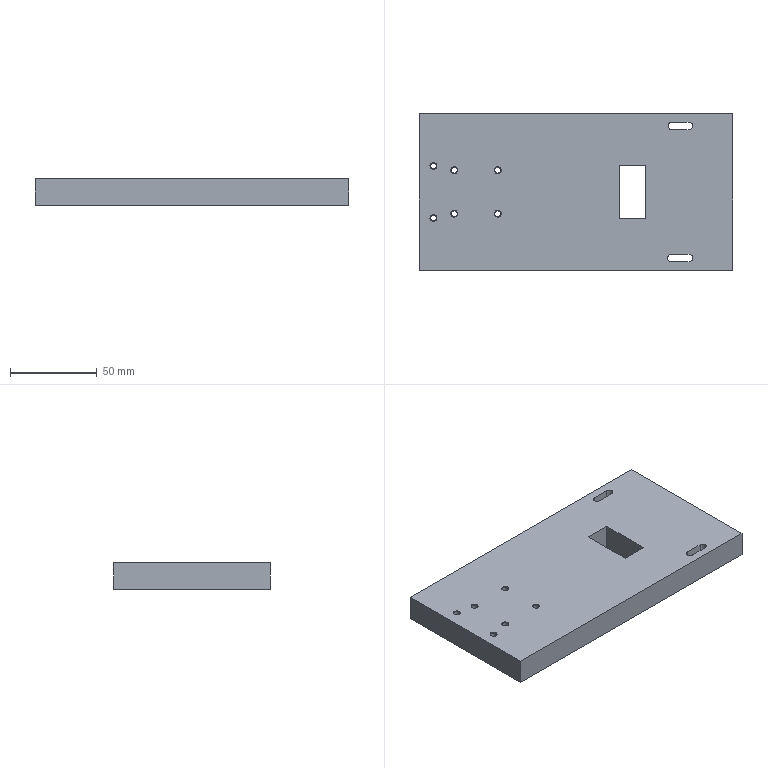Part | NX | features SIMPLE HOLE 6, SYMBOLIC_THREAD 6, DATUM_CSYS 5, SKETCH 4, EXTRUDE 3, HOLE PACKAGE 1 | 1 solid | 36 faces | box 180 x 90 x 15 mm | volume 233788 mm3 | plane 14 | cone 12 | cylinder 10 | commonest cylinder face diameters 3.3 x6 4.2 x4
STEP:
#1=CARTESIAN_POINT('',(-90.,45.,0.));
#2=VERTEX_POINT('',#1);
#3=CARTESIAN_POINT('',(-90.,-45.,0.));
#4=VERTEX_POINT('',#3);
#5=CARTESIAN_POINT('',(-90.,45.,0.));
#6=DIRECTION('',(0.,-1.,0.));
#7=VECTOR('',#6,1000.);
#8=LINE('',#5,#7);
#9=EDGE_CURVE('',#2,#4,#8,.T.);
#10=ORIENTED_EDGE('',*,*,#9,.T.);
#11=CARTESIAN_POINT('',(-90.,-45.,15.));
#12=VERTEX_POINT('',#11);
#13=CARTESIAN_POINT('',(-90.,-45.,15.));
#14=DIRECTION('',(0.,0.,-1.));
#15=VECTOR('',#14,1000.);
#16=LINE('',#13,#15);
#17=EDGE_CURVE('',#12,#4,#16,.T.);
#18=ORIENTED_EDGE('',*,*,#17,.F.);
#19=CARTESIAN_POINT('',(-90.,45.,15.));
#20=VERTEX_POINT('',#19);
#21=CARTESIAN_POINT('',(-90.,45.,15.));
#22=DIRECTION('',(0.,-1.,0.));
#23=VECTOR('',#22,1000.);
#24=LINE('',#21,#23);
#25=EDGE_CURVE('',#20,#12,#24,.T.);
#26=ORIENTED_EDGE('',*,*,#25,.F.);
#27=CARTESIAN_POINT('',(-90.,45.,15.));
#28=DIRECTION('',(0.,0.,-1.));
#29=VECTOR('',#28,1000.);
#30=LINE('',#27,#29);
#31=EDGE_CURVE('',#20,#2,#30,.T.);
#32=ORIENTED_EDGE('',*,*,#31,.T.);
#33=EDGE_LOOP('',(#10,#18,#26,#32));
#34=FACE_BOUND('',#33,.T.);
#35=CARTESIAN_POINT('',(-90.,45.,15.));
#36=DIRECTION('',(1.,0.,0.));
#37=DIRECTION('',(0.,0.,-1.));
#38=AXIS2_PLACEMENT_3D('',#35,#36,#37);
#39=PLANE('',#38);
#40=ADVANCED_FACE('',(#34),#39,.F.);
#41=CARTESIAN_POINT('',(90.,-45.,0.));
#42=VERTEX_POINT('',#41);
#43=CARTESIAN_POINT('',(-90.,-45.,0.));
#44=DIRECTION('',(1.,0.,0.));
#45=VECTOR('',#44,1000.);
#46=LINE('',#43,#45);
#47=EDGE_CURVE('',#4,#42,#46,.T.);
#48=ORIENTED_EDGE('',*,*,#47,.T.);
#49=CARTESIAN_POINT('',(90.,-45.,15.));
#50=VERTEX_POINT('',#49);
#51=CARTESIAN_POINT('',(90.,-45.,15.));
#52=DIRECTION('',(0.,0.,-1.));
#53=VECTOR('',#52,1000.);
#54=LINE('',#51,#53);
#55=EDGE_CURVE('',#50,#42,#54,.T.);
#56=ORIENTED_EDGE('',*,*,#55,.F.);
#57=CARTESIAN_POINT('',(-90.,-45.,15.));
#58=DIRECTION('',(1.,0.,0.));
#59=VECTOR('',#58,1000.);
#60=LINE('',#57,#59);
#61=EDGE_CURVE('',#12,#50,#60,.T.);
#62=ORIENTED_EDGE('',*,*,#61,.F.);
#63=ORIENTED_EDGE('',*,*,#17,.T.);
#64=EDGE_LOOP('',(#48,#56,#62,#63));
#65=FACE_BOUND('',#64,.T.);
#66=CARTESIAN_POINT('',(-90.,-45.,15.));
#67=DIRECTION('',(0.,1.,0.));
#68=DIRECTION('',(0.,0.,1.));
#69=AXIS2_PLACEMENT_3D('',#66,#67,#68);
#70=PLANE('',#69);
#71=ADVANCED_FACE('',(#65),#70,.F.);
#72=CARTESIAN_POINT('',(90.,45.,0.));
#73=VERTEX_POINT('',#72);
#74=CARTESIAN_POINT('',(90.,-45.,0.));
#75=DIRECTION('',(0.,1.,0.));
#76=VECTOR('',#75,1000.);
#77=LINE('',#74,#76);
#78=EDGE_CURVE('',#42,#73,#77,.T.);
#79=ORIENTED_EDGE('',*,*,#78,.T.);
#80=CARTESIAN_POINT('',(90.,45.,15.));
#81=VERTEX_POINT('',#80);
#82=CARTESIAN_POINT('',(90.,45.,15.));
#83=DIRECTION('',(0.,0.,-1.));
#84=VECTOR('',#83,1000.);
#85=LINE('',#82,#84);
#86=EDGE_CURVE('',#81,#73,#85,.T.);
#87=ORIENTED_EDGE('',*,*,#86,.F.);
#88=CARTESIAN_POINT('',(90.,-45.,15.));
#89=DIRECTION('',(0.,1.,0.));
#90=VECTOR('',#89,1000.);
#91=LINE('',#88,#90);
#92=EDGE_CURVE('',#50,#81,#91,.T.);
#93=ORIENTED_EDGE('',*,*,#92,.F.);
#94=ORIENTED_EDGE('',*,*,#55,.T.);
#95=EDGE_LOOP('',(#79,#87,#93,#94));
#96=FACE_BOUND('',#95,.T.);
#97=CARTESIAN_POINT('',(90.,-45.,15.));
#98=DIRECTION('',(-1.,0.,0.));
#99=DIRECTION('',(0.,0.,1.));
#100=AXIS2_PLACEMENT_3D('',#97,#98,#99);
#101=PLANE('',#100);
#102=ADVANCED_FACE('',(#96),#101,.F.);
#103=CARTESIAN_POINT('',(90.,45.,0.));
#104=DIRECTION('',(-1.,0.,0.));
#105=VECTOR('',#104,1000.);
#106=LINE('',#103,#105);
#107=EDGE_CURVE('',#73,#2,#106,.T.);
#108=ORIENTED_EDGE('',*,*,#107,.T.);
#109=ORIENTED_EDGE('',*,*,#31,.F.);
#110=CARTESIAN_POINT('',(90.,45.,15.));
#111=DIRECTION('',(-1.,0.,0.));
#112=VECTOR('',#111,1000.);
#113=LINE('',#110,#112);
#114=EDGE_CURVE('',#81,#20,#113,.T.);
#115=ORIENTED_EDGE('',*,*,#114,.F.);
#116=ORIENTED_EDGE('',*,*,#86,.T.);
#117=EDGE_LOOP('',(#108,#109,#115,#116));
#118=FACE_BOUND('',#117,.T.);
#119=CARTESIAN_POINT('',(90.,45.,15.));
#120=DIRECTION('',(0.,-1.,0.));
#121=DIRECTION('',(0.,0.,-1.));
#122=AXIS2_PLACEMENT_3D('',#119,#120,#121);
#123=PLANE('',#122);
#124=ADVANCED_FACE('',(#118),#123,.F.);
#125=CARTESIAN_POINT('',(25.,15.,15.));
#126=VERTEX_POINT('',#125);
#127=CARTESIAN_POINT('',(25.,-15.,15.));
#128=VERTEX_POINT('',#127);
#129=CARTESIAN_POINT('',(25.,15.,15.));
#130=DIRECTION('',(0.,-1.,0.));
#131=VECTOR('',#130,1000.);
#132=LINE('',#129,#131);
#133=EDGE_CURVE('',#126,#128,#132,.T.);
#134=ORIENTED_EDGE('',*,*,#133,.F.);
#135=CARTESIAN_POINT('',(40.,15.,15.));
#136=VERTEX_POINT('',#135);
#137=CARTESIAN_POINT('',(40.,15.,15.));
#138=DIRECTION('',(-1.,0.,0.));
#139=VECTOR('',#138,1000.);
#140=LINE('',#137,#139);
#141=EDGE_CURVE('',#136,#126,#140,.T.);
#142=ORIENTED_EDGE('',*,*,#141,.F.);
#143=CARTESIAN_POINT('',(40.,-15.,15.));
#144=VERTEX_POINT('',#143);
#145=CARTESIAN_POINT('',(40.,-15.,15.));
#146=DIRECTION('',(0.,1.,0.));
#147=VECTOR('',#146,1000.);
#148=LINE('',#145,#147);
#149=EDGE_CURVE('',#144,#136,#148,.T.);
#150=ORIENTED_EDGE('',*,*,#149,.F.);
#151=CARTESIAN_POINT('',(25.,-15.,15.));
#152=DIRECTION('',(1.,0.,0.));
#153=VECTOR('',#152,1000.);
#154=LINE('',#151,#153);
#155=EDGE_CURVE('',#128,#144,#154,.T.);
#156=ORIENTED_EDGE('',*,*,#155,.F.);
#157=EDGE_LOOP('',(#134,#142,#150,#156));
#158=FACE_BOUND('',#157,.T.);
#159=CARTESIAN_POINT('',(-80.,15.,15.));
#160=VERTEX_POINT('',#159);
#161=CARTESIAN_POINT('',(-82.,15.,15.));
#162=DIRECTION('',(0.,0.,1.));
#163=DIRECTION('',(1.,0.,0.));
#164=AXIS2_PLACEMENT_3D('',#161,#162,#163);
#165=CIRCLE('',#164,2.);
#166=EDGE_CURVE('',#160,#160,#165,.F.);
#167=ORIENTED_EDGE('',*,*,#166,.T.);
#168=EDGE_LOOP('',(#167));
#169=FACE_BOUND('',#168,.T.);
#170=CARTESIAN_POINT('',(-80.,-15.,15.));
#171=VERTEX_POINT('',#170);
#172=CARTESIAN_POINT('',(-82.,-15.,15.));
#173=DIRECTION('',(0.,0.,1.));
#174=DIRECTION('',(1.,0.,0.));
#175=AXIS2_PLACEMENT_3D('',#172,#173,#174);
#176=CIRCLE('',#175,2.);
#177=EDGE_CURVE('',#171,#171,#176,.F.);
#178=ORIENTED_EDGE('',*,*,#177,.T.);
#179=EDGE_LOOP('',(#178));
#180=FACE_BOUND('',#179,.T.);
#181=CARTESIAN_POINT('',(-43.,12.5,15.));
#182=VERTEX_POINT('',#181);
#183=CARTESIAN_POINT('',(-45.,12.5,15.));
#184=DIRECTION('',(0.,0.,1.));
#185=DIRECTION('',(1.,0.,0.));
#186=AXIS2_PLACEMENT_3D('',#183,#184,#185);
#187=CIRCLE('',#186,2.);
#188=EDGE_CURVE('',#182,#182,#187,.F.);
#189=ORIENTED_EDGE('',*,*,#188,.T.);
#190=EDGE_LOOP('',(#189));
#191=FACE_BOUND('',#190,.T.);
#192=CARTESIAN_POINT('',(-43.,-12.5,15.));
#193=VERTEX_POINT('',#192);
#194=CARTESIAN_POINT('',(-45.,-12.5,15.));
#195=DIRECTION('',(0.,0.,1.));
#196=DIRECTION('',(1.,0.,0.));
#197=AXIS2_PLACEMENT_3D('',#194,#195,#196);
#198=CIRCLE('',#197,2.);
#199=EDGE_CURVE('',#193,#193,#198,.F.);
#200=ORIENTED_EDGE('',*,*,#199,.T.);
#201=EDGE_LOOP('',(#200));
#202=FACE_BOUND('',#201,.T.);
#203=CARTESIAN_POINT('',(-68.,12.5,15.));
#204=VERTEX_POINT('',#203);
#205=CARTESIAN_POINT('',(-70.,12.5,15.));
#206=DIRECTION('',(0.,0.,1.));
#207=DIRECTION('',(1.,0.,0.));
#208=AXIS2_PLACEMENT_3D('',#205,#206,#207);
#209=CIRCLE('',#208,2.);
#210=EDGE_CURVE('',#204,#204,#209,.F.);
#211=ORIENTED_EDGE('',*,*,#210,.T.);
#212=EDGE_LOOP('',(#211));
#213=FACE_BOUND('',#212,.T.);
#214=CARTESIAN_POINT('',(-68.,-12.5,15.));
#215=VERTEX_POINT('',#214);
#216=CARTESIAN_POINT('',(-70.,-12.5,15.));
#217=DIRECTION('',(0.,0.,1.));
#218=DIRECTION('',(1.,0.,0.));
#219=AXIS2_PLACEMENT_3D('',#216,#217,#218);
#220=CIRCLE('',#219,2.);
#221=EDGE_CURVE('',#215,#215,#220,.F.);
#222=ORIENTED_EDGE('',*,*,#221,.T.);
#223=EDGE_LOOP('',(#222));
#224=FACE_BOUND('',#223,.T.);
#225=CARTESIAN_POINT('',(55.,40.1,15.));
#226=VERTEX_POINT('',#225);
#227=CARTESIAN_POINT('',(55.,35.9,15.));
#228=VERTEX_POINT('',#227);
#229=CARTESIAN_POINT('',(55.,38.,15.));
#230=DIRECTION('',(0.,0.,1.));
#231=DIRECTION('',(0.,1.,0.));
#232=AXIS2_PLACEMENT_3D('',#229,#230,#231);
#233=CIRCLE('',#232,2.1);
#234=EDGE_CURVE('',#226,#228,#233,.T.);
#235=ORIENTED_EDGE('',*,*,#234,.F.);
#236=CARTESIAN_POINT('',(65.,40.1,15.));
#237=VERTEX_POINT('',#236);
#238=CARTESIAN_POINT('',(65.,40.1,15.));
#239=DIRECTION('',(-1.,0.,0.));
#240=VECTOR('',#239,1000.);
#241=LINE('',#238,#240);
#242=EDGE_CURVE('',#237,#226,#241,.T.);
#243=ORIENTED_EDGE('',*,*,#242,.F.);
#244=CARTESIAN_POINT('',(65.,35.9,15.));
#245=VERTEX_POINT('',#244);
#246=CARTESIAN_POINT('',(65.,38.,15.));
#247=DIRECTION('',(0.,0.,1.));
#248=DIRECTION('',(0.,1.,0.));
#249=AXIS2_PLACEMENT_3D('',#246,#247,#248);
#250=CIRCLE('',#249,2.1);
#251=EDGE_CURVE('',#245,#237,#250,.T.);
#252=ORIENTED_EDGE('',*,*,#251,.F.);
#253=CARTESIAN_POINT('',(55.,35.9,15.));
#254=DIRECTION('',(1.,0.,0.));
#255=VECTOR('',#254,1000.);
#256=LINE('',#253,#255);
#257=EDGE_CURVE('',#228,#245,#256,.T.);
#258=ORIENTED_EDGE('',*,*,#257,.F.);
#259=EDGE_LOOP('',(#235,#243,#252,#258));
#260=FACE_BOUND('',#259,.T.);
#261=CARTESIAN_POINT('',(54.858,-35.9,15.));
#262=VERTEX_POINT('',#261);
#263=CARTESIAN_POINT('',(54.858,-40.1,15.));
#264=VERTEX_POINT('',#263);
#265=CARTESIAN_POINT('',(54.858,-38.,15.));
#266=DIRECTION('',(0.,0.,1.));
#267=DIRECTION('',(0.,1.,0.));
#268=AXIS2_PLACEMENT_3D('',#265,#266,#267);
#269=CIRCLE('',#268,2.1);
#270=EDGE_CURVE('',#262,#264,#269,.T.);
#271=ORIENTED_EDGE('',*,*,#270,.F.);
#272=CARTESIAN_POINT('',(65.,-35.9,15.));
#273=VERTEX_POINT('',#272);
#274=CARTESIAN_POINT('',(65.,-35.9,15.));
#275=DIRECTION('',(-1.,0.,0.));
#276=VECTOR('',#275,1000.);
#277=LINE('',#274,#276);
#278=EDGE_CURVE('',#273,#262,#277,.T.);
#279=ORIENTED_EDGE('',*,*,#278,.F.);
#280=CARTESIAN_POINT('',(65.,-40.1,15.));
#281=VERTEX_POINT('',#280);
#282=CARTESIAN_POINT('',(65.,-38.,15.));
#283=DIRECTION('',(0.,0.,1.));
#284=DIRECTION('',(0.,1.,0.));
#285=AXIS2_PLACEMENT_3D('',#282,#283,#284);
#286=CIRCLE('',#285,2.1);
#287=EDGE_CURVE('',#281,#273,#286,.T.);
#288=ORIENTED_EDGE('',*,*,#287,.F.);
#289=CARTESIAN_POINT('',(54.858,-40.1,15.));
#290=DIRECTION('',(1.,0.,0.));
#291=VECTOR('',#290,1000.);
#292=LINE('',#289,#291);
#293=EDGE_CURVE('',#264,#281,#292,.T.);
#294=ORIENTED_EDGE('',*,*,#293,.F.);
#295=EDGE_LOOP('',(#271,#279,#288,#294));
#296=FACE_BOUND('',#295,.T.);
#297=ORIENTED_EDGE('',*,*,#25,.T.);
#298=ORIENTED_EDGE('',*,*,#61,.T.);
#299=ORIENTED_EDGE('',*,*,#92,.T.);
#300=ORIENTED_EDGE('',*,*,#114,.T.);
#301=EDGE_LOOP('',(#297,#298,#299,#300));
#302=FACE_BOUND('',#301,.T.);
#303=CARTESIAN_POINT('',(0.,0.,15.));
#304=DIRECTION('',(0.,0.,1.));
#305=DIRECTION('',(1.,0.,0.));
#306=AXIS2_PLACEMENT_3D('',#303,#304,#305);
#307=PLANE('',#306);
#308=ADVANCED_FACE('',(#158,#169,#180,#191,#202,#213,#224,#260,#296,#302),#307,.T.);
#309=CARTESIAN_POINT('',(40.,15.,0.));
#310=VERTEX_POINT('',#309);
#311=CARTESIAN_POINT('',(25.,15.,0.));
#312=VERTEX_POINT('',#311);
#313=CARTESIAN_POINT('',(40.,15.,0.));
#314=DIRECTION('',(-1.,0.,0.));
#315=VECTOR('',#314,1000.);
#316=LINE('',#313,#315);
#317=EDGE_CURVE('',#310,#312,#316,.T.);
#318=ORIENTED_EDGE('',*,*,#317,.T.);
#319=CARTESIAN_POINT('',(25.,-15.,0.));
#320=VERTEX_POINT('',#319);
#321=CARTESIAN_POINT('',(25.,15.,0.));
#322=DIRECTION('',(0.,-1.,0.));
#323=VECTOR('',#322,1000.);
#324=LINE('',#321,#323);
#325=EDGE_CURVE('',#312,#320,#324,.T.);
#326=ORIENTED_EDGE('',*,*,#325,.T.);
#327=CARTESIAN_POINT('',(40.,-15.,0.));
#328=VERTEX_POINT('',#327);
#329=CARTESIAN_POINT('',(25.,-15.,0.));
#330=DIRECTION('',(1.,0.,0.));
#331=VECTOR('',#330,1000.);
#332=LINE('',#329,#331);
#333=EDGE_CURVE('',#320,#328,#332,.T.);
#334=ORIENTED_EDGE('',*,*,#333,.T.);
#335=CARTESIAN_POINT('',(40.,-15.,0.));
#336=DIRECTION('',(0.,1.,0.));
#337=VECTOR('',#336,1000.);
#338=LINE('',#335,#337);
#339=EDGE_CURVE('',#328,#310,#338,.T.);
#340=ORIENTED_EDGE('',*,*,#339,.T.);
#341=EDGE_LOOP('',(#318,#326,#334,#340));
#342=FACE_BOUND('',#341,.T.);
#343=CARTESIAN_POINT('',(-80.,15.,0.));
#344=VERTEX_POINT('',#343);
#345=CARTESIAN_POINT('',(-82.,15.,0.));
#346=DIRECTION('',(0.,0.,1.));
#347=DIRECTION('',(1.,0.,0.));
#348=AXIS2_PLACEMENT_3D('',#345,#346,#347);
#349=CIRCLE('',#348,2.);
#350=EDGE_CURVE('',#344,#344,#349,.T.);
#351=ORIENTED_EDGE('',*,*,#350,.T.);
#352=EDGE_LOOP('',(#351));
#353=FACE_BOUND('',#352,.T.);
#354=CARTESIAN_POINT('',(-80.,-15.,0.));
#355=VERTEX_POINT('',#354);
#356=CARTESIAN_POINT('',(-82.,-15.,0.));
#357=DIRECTION('',(0.,0.,1.));
#358=DIRECTION('',(1.,0.,0.));
#359=AXIS2_PLACEMENT_3D('',#356,#357,#358);
#360=CIRCLE('',#359,2.);
#361=EDGE_CURVE('',#355,#355,#360,.T.);
#362=ORIENTED_EDGE('',*,*,#361,.T.);
#363=EDGE_LOOP('',(#362));
#364=FACE_BOUND('',#363,.T.);
#365=CARTESIAN_POINT('',(-43.,12.5,0.));
#366=VERTEX_POINT('',#365);
#367=CARTESIAN_POINT('',(-45.,12.5,0.));
#368=DIRECTION('',(0.,0.,1.));
#369=DIRECTION('',(1.,0.,0.));
#370=AXIS2_PLACEMENT_3D('',#367,#368,#369);
#371=CIRCLE('',#370,2.);
#372=EDGE_CURVE('',#366,#366,#371,.T.);
#373=ORIENTED_EDGE('',*,*,#372,.T.);
#374=EDGE_LOOP('',(#373));
#375=FACE_BOUND('',#374,.T.);
#376=CARTESIAN_POINT('',(-43.,-12.5,0.));
#377=VERTEX_POINT('',#376);
#378=CARTESIAN_POINT('',(-45.,-12.5,0.));
#379=DIRECTION('',(0.,0.,1.));
#380=DIRECTION('',(1.,0.,0.));
#381=AXIS2_PLACEMENT_3D('',#378,#379,#380);
#382=CIRCLE('',#381,2.);
#383=EDGE_CURVE('',#377,#377,#382,.T.);
#384=ORIENTED_EDGE('',*,*,#383,.T.);
#385=EDGE_LOOP('',(#384));
#386=FACE_BOUND('',#385,.T.);
#387=CARTESIAN_POINT('',(-68.,12.5,0.));
#388=VERTEX_POINT('',#387);
#389=CARTESIAN_POINT('',(-70.,12.5,0.));
#390=DIRECTION('',(0.,0.,1.));
#391=DIRECTION('',(1.,0.,0.));
#392=AXIS2_PLACEMENT_3D('',#389,#390,#391);
#393=CIRCLE('',#392,2.);
#394=EDGE_CURVE('',#388,#388,#393,.T.);
#395=ORIENTED_EDGE('',*,*,#394,.T.);
#396=EDGE_LOOP('',(#395));
#397=FACE_BOUND('',#396,.T.);
#398=CARTESIAN_POINT('',(-68.,-12.5,0.));
#399=VERTEX_POINT('',#398);
#400=CARTESIAN_POINT('',(-70.,-12.5,0.));
#401=DIRECTION('',(0.,0.,1.));
#402=DIRECTION('',(1.,0.,0.));
#403=AXIS2_PLACEMENT_3D('',#400,#401,#402);
#404=CIRCLE('',#403,2.);
#405=EDGE_CURVE('',#399,#399,#404,.T.);
#406=ORIENTED_EDGE('',*,*,#405,.T.);
#407=EDGE_LOOP('',(#406));
#408=FACE_BOUND('',#407,.T.);
#409=CARTESIAN_POINT('',(65.,40.1,0.));
#410=VERTEX_POINT('',#409);
#411=CARTESIAN_POINT('',(55.,40.1,0.));
#412=VERTEX_POINT('',#411);
#413=CARTESIAN_POINT('',(65.,40.1,0.));
#414=DIRECTION('',(-1.,0.,0.));
#415=VECTOR('',#414,1000.);
#416=LINE('',#413,#415);
#417=EDGE_CURVE('',#410,#412,#416,.T.);
#418=ORIENTED_EDGE('',*,*,#417,.T.);
#419=CARTESIAN_POINT('',(55.,35.9,0.));
#420=VERTEX_POINT('',#419);
#421=CARTESIAN_POINT('',(55.,38.,0.));
#422=DIRECTION('',(0.,0.,1.));
#423=DIRECTION('',(0.,1.,0.));
#424=AXIS2_PLACEMENT_3D('',#421,#422,#423);
#425=CIRCLE('',#424,2.1);
#426=EDGE_CURVE('',#412,#420,#425,.T.);
#427=ORIENTED_EDGE('',*,*,#426,.T.);
#428=CARTESIAN_POINT('',(65.,35.9,0.));
#429=VERTEX_POINT('',#428);
#430=CARTESIAN_POINT('',(55.,35.9,0.));
#431=DIRECTION('',(1.,0.,0.));
#432=VECTOR('',#431,1000.);
#433=LINE('',#430,#432);
#434=EDGE_CURVE('',#420,#429,#433,.T.);
#435=ORIENTED_EDGE('',*,*,#434,.T.);
#436=CARTESIAN_POINT('',(65.,38.,0.));
#437=DIRECTION('',(0.,0.,1.));
#438=DIRECTION('',(0.,1.,0.));
#439=AXIS2_PLACEMENT_3D('',#436,#437,#438);
#440=CIRCLE('',#439,2.1);
#441=EDGE_CURVE('',#429,#410,#440,.T.);
#442=ORIENTED_EDGE('',*,*,#441,.T.);
#443=EDGE_LOOP('',(#418,#427,#435,#442));
#444=FACE_BOUND('',#443,.T.);
#445=CARTESIAN_POINT('',(65.,-35.9,0.));
#446=VERTEX_POINT('',#445);
#447=CARTESIAN_POINT('',(54.858,-35.9,0.));
#448=VERTEX_POINT('',#447);
#449=CARTESIAN_POINT('',(65.,-35.9,0.));
#450=DIRECTION('',(-1.,0.,0.));
#451=VECTOR('',#450,1000.);
#452=LINE('',#449,#451);
#453=EDGE_CURVE('',#446,#448,#452,.T.);
#454=ORIENTED_EDGE('',*,*,#453,.T.);
#455=CARTESIAN_POINT('',(54.858,-40.1,0.));
#456=VERTEX_POINT('',#455);
#457=CARTESIAN_POINT('',(54.858,-38.,0.));
#458=DIRECTION('',(0.,0.,1.));
#459=DIRECTION('',(0.,1.,0.));
#460=AXIS2_PLACEMENT_3D('',#457,#458,#459);
#461=CIRCLE('',#460,2.1);
#462=EDGE_CURVE('',#448,#456,#461,.T.);
#463=ORIENTED_EDGE('',*,*,#462,.T.);
#464=CARTESIAN_POINT('',(65.,-40.1,0.));
#465=VERTEX_POINT('',#464);
#466=CARTESIAN_POINT('',(54.858,-40.1,0.));
#467=DIRECTION('',(1.,0.,0.));
#468=VECTOR('',#467,1000.);
#469=LINE('',#466,#468);
#470=EDGE_CURVE('',#456,#465,#469,.T.);
#471=ORIENTED_EDGE('',*,*,#470,.T.);
#472=CARTESIAN_POINT('',(65.,-38.,0.));
#473=DIRECTION('',(0.,0.,1.));
#474=DIRECTION('',(0.,1.,0.));
#475=AXIS2_PLACEMENT_3D('',#472,#473,#474);
#476=CIRCLE('',#475,2.1);
#477=EDGE_CURVE('',#465,#446,#476,.T.);
#478=ORIENTED_EDGE('',*,*,#477,.T.);
#479=EDGE_LOOP('',(#454,#463,#471,#478));
#480=FACE_BOUND('',#479,.T.);
#481=ORIENTED_EDGE('',*,*,#9,.F.);
#482=ORIENTED_EDGE('',*,*,#107,.F.);
#483=ORIENTED_EDGE('',*,*,#78,.F.);
#484=ORIENTED_EDGE('',*,*,#47,.F.);
#485=EDGE_LOOP('',(#481,#482,#483,#484));
#486=FACE_BOUND('',#485,.T.);
#487=CARTESIAN_POINT('',(0.,0.,0.));
#488=DIRECTION('',(0.,0.,1.));
#489=DIRECTION('',(1.,0.,0.));
#490=AXIS2_PLACEMENT_3D('',#487,#488,#489);
#491=PLANE('',#490);
#492=ADVANCED_FACE('',(#342,#353,#364,#375,#386,#397,#408,#444,#480,#486),#491,.F.);
#493=ORIENTED_EDGE('',*,*,#270,.T.);
#494=CARTESIAN_POINT('',(54.858,-40.1,0.));
#495=DIRECTION('',(0.,0.,1.));
#496=VECTOR('',#495,1000.);
#497=LINE('',#494,#496);
#498=EDGE_CURVE('',#264,#456,#497,.F.);
#499=ORIENTED_EDGE('',*,*,#498,.T.);
#500=ORIENTED_EDGE('',*,*,#462,.F.);
#501=CARTESIAN_POINT('',(54.858,-35.9,0.));
#502=DIRECTION('',(0.,0.,1.));
#503=VECTOR('',#502,1000.);
#504=LINE('',#501,#503);
#505=EDGE_CURVE('',#262,#448,#504,.F.);
#506=ORIENTED_EDGE('',*,*,#505,.F.);
#507=EDGE_LOOP('',(#493,#499,#500,#506));
#508=FACE_BOUND('',#507,.T.);
#509=CARTESIAN_POINT('',(54.858,-38.,0.));
#510=DIRECTION('',(0.,0.,1.));
#511=DIRECTION('',(1.,0.,0.));
#512=AXIS2_PLACEMENT_3D('',#509,#510,#511);
#513=CYLINDRICAL_SURFACE('',#512,2.1);
#514=ADVANCED_FACE('',(#508),#513,.F.);
#515=ORIENTED_EDGE('',*,*,#293,.T.);
#516=CARTESIAN_POINT('',(65.,-40.1,0.));
#517=DIRECTION('',(0.,0.,1.));
#518=VECTOR('',#517,1000.);
#519=LINE('',#516,#518);
#520=EDGE_CURVE('',#281,#465,#519,.F.);
#521=ORIENTED_EDGE('',*,*,#520,.T.);
#522=ORIENTED_EDGE('',*,*,#470,.F.);
#523=ORIENTED_EDGE('',*,*,#498,.F.);
#524=EDGE_LOOP('',(#515,#521,#522,#523));
#525=FACE_BOUND('',#524,.T.);
#526=CARTESIAN_POINT('',(54.858,-40.1,0.));
#527=DIRECTION('',(0.,-1.,0.));
#528=DIRECTION('',(0.,0.,-1.));
#529=AXIS2_PLACEMENT_3D('',#526,#527,#528);
#530=PLANE('',#529);
#531=ADVANCED_FACE('',(#525),#530,.F.);
#532=ORIENTED_EDGE('',*,*,#287,.T.);
#533=CARTESIAN_POINT('',(65.,-35.9,0.));
#534=DIRECTION('',(0.,0.,1.));
#535=VECTOR('',#534,1000.);
#536=LINE('',#533,#535);
#537=EDGE_CURVE('',#273,#446,#536,.F.);
#538=ORIENTED_EDGE('',*,*,#537,.T.);
#539=ORIENTED_EDGE('',*,*,#477,.F.);
#540=ORIENTED_EDGE('',*,*,#520,.F.);
#541=EDGE_LOOP('',(#532,#538,#539,#540));
#542=FACE_BOUND('',#541,.T.);
#543=CARTESIAN_POINT('',(65.,-38.,0.));
#544=DIRECTION('',(0.,0.,1.));
#545=DIRECTION('',(1.,0.,0.));
#546=AXIS2_PLACEMENT_3D('',#543,#544,#545);
#547=CYLINDRICAL_SURFACE('',#546,2.1);
#548=ADVANCED_FACE('',(#542),#547,.F.);
#549=ORIENTED_EDGE('',*,*,#278,.T.);
#550=ORIENTED_EDGE('',*,*,#505,.T.);
#551=ORIENTED_EDGE('',*,*,#453,.F.);
#552=ORIENTED_EDGE('',*,*,#537,.F.);
#553=EDGE_LOOP('',(#549,#550,#551,#552));
#554=FACE_BOUND('',#553,.T.);
#555=CARTESIAN_POINT('',(65.,-35.9,0.));
#556=DIRECTION('',(0.,1.,0.));
#557=DIRECTION('',(0.,0.,1.));
#558=AXIS2_PLACEMENT_3D('',#555,#556,#557);
#559=PLANE('',#558);
#560=ADVANCED_FACE('',(#554),#559,.F.);
#561=ORIENTED_EDGE('',*,*,#234,.T.);
#562=CARTESIAN_POINT('',(55.,35.9,0.));
#563=DIRECTION('',(0.,0.,1.));
#564=VECTOR('',#563,1000.);
#565=LINE('',#562,#564);
#566=EDGE_CURVE('',#228,#420,#565,.F.);
#567=ORIENTED_EDGE('',*,*,#566,.T.);
#568=ORIENTED_EDGE('',*,*,#426,.F.);
#569=CARTESIAN_POINT('',(55.,40.1,0.));
#570=DIRECTION('',(0.,0.,1.));
#571=VECTOR('',#570,1000.);
#572=LINE('',#569,#571);
#573=EDGE_CURVE('',#226,#412,#572,.F.);
#574=ORIENTED_EDGE('',*,*,#573,.F.);
#575=EDGE_LOOP('',(#561,#567,#568,#574));
#576=FACE_BOUND('',#575,.T.);
#577=CARTESIAN_POINT('',(55.,38.,0.));
#578=DIRECTION('',(0.,0.,1.));
#579=DIRECTION('',(1.,0.,0.));
#580=AXIS2_PLACEMENT_3D('',#577,#578,#579);
#581=CYLINDRICAL_SURFACE('',#580,2.1);
#582=ADVANCED_FACE('',(#576),#581,.F.);
#583=ORIENTED_EDGE('',*,*,#257,.T.);
#584=CARTESIAN_POINT('',(65.,35.9,0.));
#585=DIRECTION('',(0.,0.,1.));
#586=VECTOR('',#585,1000.);
#587=LINE('',#584,#586);
#588=EDGE_CURVE('',#245,#429,#587,.F.);
#589=ORIENTED_EDGE('',*,*,#588,.T.);
#590=ORIENTED_EDGE('',*,*,#434,.F.);
#591=ORIENTED_EDGE('',*,*,#566,.F.);
#592=EDGE_LOOP('',(#583,#589,#590,#591));
#593=FACE_BOUND('',#592,.T.);
#594=CARTESIAN_POINT('',(55.,35.9,0.));
#595=DIRECTION('',(0.,-1.,0.));
#596=DIRECTION('',(1.,0.,0.));
#597=AXIS2_PLACEMENT_3D('',#594,#595,#596);
#598=PLANE('',#597);
#599=ADVANCED_FACE('',(#593),#598,.F.);
#600=ORIENTED_EDGE('',*,*,#251,.T.);
#601=CARTESIAN_POINT('',(65.,40.1,0.));
#602=DIRECTION('',(0.,0.,1.));
#603=VECTOR('',#602,1000.);
#604=LINE('',#601,#603);
#605=EDGE_CURVE('',#237,#410,#604,.F.);
#606=ORIENTED_EDGE('',*,*,#605,.T.);
#607=ORIENTED_EDGE('',*,*,#441,.F.);
#608=ORIENTED_EDGE('',*,*,#588,.F.);
#609=EDGE_LOOP('',(#600,#606,#607,#608));
#610=FACE_BOUND('',#609,.T.);
#611=CARTESIAN_POINT('',(65.,38.,0.));
#612=DIRECTION('',(0.,0.,1.));
#613=DIRECTION('',(1.,0.,0.));
#614=AXIS2_PLACEMENT_3D('',#611,#612,#613);
#615=CYLINDRICAL_SURFACE('',#614,2.1);
#616=ADVANCED_FACE('',(#610),#615,.F.);
#617=ORIENTED_EDGE('',*,*,#242,.T.);
#618=ORIENTED_EDGE('',*,*,#573,.T.);
#619=ORIENTED_EDGE('',*,*,#417,.F.);
#620=ORIENTED_EDGE('',*,*,#605,.F.);
#621=EDGE_LOOP('',(#617,#618,#619,#620));
#622=FACE_BOUND('',#621,.T.);
#623=CARTESIAN_POINT('',(65.,40.1,0.));
#624=DIRECTION('',(0.,1.,0.));
#625=DIRECTION('',(0.,0.,1.));
#626=AXIS2_PLACEMENT_3D('',#623,#624,#625);
#627=PLANE('',#626);
#628=ADVANCED_FACE('',(#622),#627,.F.);
#629=CARTESIAN_POINT('',(-68.35,-12.5,0.35));
#630=VERTEX_POINT('',#629);
#631=CARTESIAN_POINT('',(-70.,-12.5,0.35));
#632=DIRECTION('',(0.,0.,1.));
#633=DIRECTION('',(1.,0.,0.));
#634=AXIS2_PLACEMENT_3D('',#631,#632,#633);
#635=CIRCLE('',#634,1.65);
#636=EDGE_CURVE('',#630,#630,#635,.F.);
#637=ORIENTED_EDGE('',*,*,#636,.T.);
#638=EDGE_LOOP('',(#637));
#639=FACE_BOUND('',#638,.T.);
#640=CARTESIAN_POINT('',(-68.35,-12.5,14.65));
#641=VERTEX_POINT('',#640);
#642=CARTESIAN_POINT('',(-70.,-12.5,14.65));
#643=DIRECTION('',(0.,0.,1.));
#644=DIRECTION('',(1.,0.,0.));
#645=AXIS2_PLACEMENT_3D('',#642,#643,#644);
#646=CIRCLE('',#645,1.65);
#647=EDGE_CURVE('',#641,#641,#646,.T.);
#648=ORIENTED_EDGE('',*,*,#647,.T.);
#649=EDGE_LOOP('',(#648));
#650=FACE_BOUND('',#649,.T.);
#651=CARTESIAN_POINT('',(-70.,-12.5,15.));
#652=DIRECTION('',(0.,0.,-1.));
#653=DIRECTION('',(-1.,0.,0.));
#654=AXIS2_PLACEMENT_3D('',#651,#652,#653);
#655=CYLINDRICAL_SURFACE('',#654,1.65);
#656=ADVANCED_FACE('',(#639,#650),#655,.F.);
#657=ORIENTED_EDGE('',*,*,#647,.F.);
#658=EDGE_LOOP('',(#657));
#659=FACE_BOUND('',#658,.T.);
#660=ORIENTED_EDGE('',*,*,#221,.F.);
#661=EDGE_LOOP('',(#660));
#662=FACE_BOUND('',#661,.T.);
#663=CARTESIAN_POINT('',(-70.,-12.5,15.));
#664=DIRECTION('',(0.,0.,1.));
#665=DIRECTION('',(1.,0.,0.));
#666=AXIS2_PLACEMENT_3D('',#663,#664,#665);
#667=CONICAL_SURFACE('',#666,2.,0.7854);
#668=ADVANCED_FACE('',(#659,#662),#667,.F.);
#669=ORIENTED_EDGE('',*,*,#636,.F.);
#670=EDGE_LOOP('',(#669));
#671=FACE_BOUND('',#670,.T.);
#672=ORIENTED_EDGE('',*,*,#405,.F.);
#673=EDGE_LOOP('',(#672));
#674=FACE_BOUND('',#673,.T.);
#675=CARTESIAN_POINT('',(-70.,-12.5,0.));
#676=DIRECTION('',(0.,0.,-1.));
#677=DIRECTION('',(-1.,0.,0.));
#678=AXIS2_PLACEMENT_3D('',#675,#676,#677);
#679=CONICAL_SURFACE('',#678,2.,0.7854);
#680=ADVANCED_FACE('',(#671,#674),#679,.F.);
#681=CARTESIAN_POINT('',(-68.35,12.5,0.35));
#682=VERTEX_POINT('',#681);
#683=CARTESIAN_POINT('',(-70.,12.5,0.35));
#684=DIRECTION('',(0.,0.,1.));
#685=DIRECTION('',(1.,0.,0.));
#686=AXIS2_PLACEMENT_3D('',#683,#684,#685);
#687=CIRCLE('',#686,1.65);
#688=EDGE_CURVE('',#682,#682,#687,.F.);
#689=ORIENTED_EDGE('',*,*,#688,.T.);
#690=EDGE_LOOP('',(#689));
#691=FACE_BOUND('',#690,.T.);
#692=CARTESIAN_POINT('',(-68.35,12.5,14.65));
#693=VERTEX_POINT('',#692);
#694=CARTESIAN_POINT('',(-70.,12.5,14.65));
#695=DIRECTION('',(0.,0.,1.));
#696=DIRECTION('',(1.,0.,0.));
#697=AXIS2_PLACEMENT_3D('',#694,#695,#696);
#698=CIRCLE('',#697,1.65);
#699=EDGE_CURVE('',#693,#693,#698,.T.);
#700=ORIENTED_EDGE('',*,*,#699,.T.);
#701=EDGE_LOOP('',(#700));
#702=FACE_BOUND('',#701,.T.);
#703=CARTESIAN_POINT('',(-70.,12.5,15.));
#704=DIRECTION('',(0.,0.,-1.));
#705=DIRECTION('',(-1.,0.,0.));
#706=AXIS2_PLACEMENT_3D('',#703,#704,#705);
#707=CYLINDRICAL_SURFACE('',#706,1.65);
#708=ADVANCED_FACE('',(#691,#702),#707,.F.);
#709=ORIENTED_EDGE('',*,*,#699,.F.);
#710=EDGE_LOOP('',(#709));
#711=FACE_BOUND('',#710,.T.);
#712=ORIENTED_EDGE('',*,*,#210,.F.);
#713=EDGE_LOOP('',(#712));
#714=FACE_BOUND('',#713,.T.);
#715=CARTESIAN_POINT('',(-70.,12.5,15.));
#716=DIRECTION('',(0.,0.,1.));
#717=DIRECTION('',(1.,0.,0.));
#718=AXIS2_PLACEMENT_3D('',#715,#716,#717);
#719=CONICAL_SURFACE('',#718,2.,0.7854);
#720=ADVANCED_FACE('',(#711,#714),#719,.F.);
#721=ORIENTED_EDGE('',*,*,#688,.F.);
#722=EDGE_LOOP('',(#721));
#723=FACE_BOUND('',#722,.T.);
#724=ORIENTED_EDGE('',*,*,#394,.F.);
#725=EDGE_LOOP('',(#724));
#726=FACE_BOUND('',#725,.T.);
#727=CARTESIAN_POINT('',(-70.,12.5,0.));
#728=DIRECTION('',(0.,0.,-1.));
#729=DIRECTION('',(-1.,0.,0.));
#730=AXIS2_PLACEMENT_3D('',#727,#728,#729);
#731=CONICAL_SURFACE('',#730,2.,0.7854);
#732=ADVANCED_FACE('',(#723,#726),#731,.F.);
#733=CARTESIAN_POINT('',(-43.35,-12.5,0.35));
#734=VERTEX_POINT('',#733);
#735=CARTESIAN_POINT('',(-45.,-12.5,0.35));
#736=DIRECTION('',(0.,0.,1.));
#737=DIRECTION('',(1.,0.,0.));
#738=AXIS2_PLACEMENT_3D('',#735,#736,#737);
#739=CIRCLE('',#738,1.65);
#740=EDGE_CURVE('',#734,#734,#739,.F.);
#741=ORIENTED_EDGE('',*,*,#740,.T.);
#742=EDGE_LOOP('',(#741));
#743=FACE_BOUND('',#742,.T.);
#744=CARTESIAN_POINT('',(-43.35,-12.5,14.65));
#745=VERTEX_POINT('',#744);
#746=CARTESIAN_POINT('',(-45.,-12.5,14.65));
#747=DIRECTION('',(0.,0.,1.));
#748=DIRECTION('',(1.,0.,0.));
#749=AXIS2_PLACEMENT_3D('',#746,#747,#748);
#750=CIRCLE('',#749,1.65);
#751=EDGE_CURVE('',#745,#745,#750,.T.);
#752=ORIENTED_EDGE('',*,*,#751,.T.);
#753=EDGE_LOOP('',(#752));
#754=FACE_BOUND('',#753,.T.);
#755=CARTESIAN_POINT('',(-45.,-12.5,15.));
#756=DIRECTION('',(0.,0.,-1.));
#757=DIRECTION('',(-1.,0.,0.));
#758=AXIS2_PLACEMENT_3D('',#755,#756,#757);
#759=CYLINDRICAL_SURFACE('',#758,1.65);
#760=ADVANCED_FACE('',(#743,#754),#759,.F.);
#761=ORIENTED_EDGE('',*,*,#751,.F.);
#762=EDGE_LOOP('',(#761));
#763=FACE_BOUND('',#762,.T.);
#764=ORIENTED_EDGE('',*,*,#199,.F.);
#765=EDGE_LOOP('',(#764));
#766=FACE_BOUND('',#765,.T.);
#767=CARTESIAN_POINT('',(-45.,-12.5,15.));
#768=DIRECTION('',(0.,0.,1.));
#769=DIRECTION('',(1.,0.,0.));
#770=AXIS2_PLACEMENT_3D('',#767,#768,#769);
#771=CONICAL_SURFACE('',#770,2.,0.7854);
#772=ADVANCED_FACE('',(#763,#766),#771,.F.);
#773=ORIENTED_EDGE('',*,*,#740,.F.);
#774=EDGE_LOOP('',(#773));
#775=FACE_BOUND('',#774,.T.);
#776=ORIENTED_EDGE('',*,*,#383,.F.);
#777=EDGE_LOOP('',(#776));
#778=FACE_BOUND('',#777,.T.);
#779=CARTESIAN_POINT('',(-45.,-12.5,0.));
#780=DIRECTION('',(0.,0.,-1.));
#781=DIRECTION('',(-1.,0.,0.));
#782=AXIS2_PLACEMENT_3D('',#779,#780,#781);
#783=CONICAL_SURFACE('',#782,2.,0.7854);
#784=ADVANCED_FACE('',(#775,#778),#783,.F.);
#785=CARTESIAN_POINT('',(-43.35,12.5,0.35));
#786=VERTEX_POINT('',#785);
#787=CARTESIAN_POINT('',(-45.,12.5,0.35));
#788=DIRECTION('',(0.,0.,1.));
#789=DIRECTION('',(1.,0.,0.));
#790=AXIS2_PLACEMENT_3D('',#787,#788,#789);
#791=CIRCLE('',#790,1.65);
#792=EDGE_CURVE('',#786,#786,#791,.F.);
#793=ORIENTED_EDGE('',*,*,#792,.T.);
#794=EDGE_LOOP('',(#793));
#795=FACE_BOUND('',#794,.T.);
#796=CARTESIAN_POINT('',(-43.35,12.5,14.65));
#797=VERTEX_POINT('',#796);
#798=CARTESIAN_POINT('',(-45.,12.5,14.65));
#799=DIRECTION('',(0.,0.,1.));
#800=DIRECTION('',(1.,0.,0.));
#801=AXIS2_PLACEMENT_3D('',#798,#799,#800);
#802=CIRCLE('',#801,1.65);
#803=EDGE_CURVE('',#797,#797,#802,.T.);
#804=ORIENTED_EDGE('',*,*,#803,.T.);
#805=EDGE_LOOP('',(#804));
#806=FACE_BOUND('',#805,.T.);
#807=CARTESIAN_POINT('',(-45.,12.5,15.));
#808=DIRECTION('',(0.,0.,-1.));
#809=DIRECTION('',(-1.,0.,0.));
#810=AXIS2_PLACEMENT_3D('',#807,#808,#809);
#811=CYLINDRICAL_SURFACE('',#810,1.65);
#812=ADVANCED_FACE('',(#795,#806),#811,.F.);
#813=ORIENTED_EDGE('',*,*,#803,.F.);
#814=EDGE_LOOP('',(#813));
#815=FACE_BOUND('',#814,.T.);
#816=ORIENTED_EDGE('',*,*,#188,.F.);
#817=EDGE_LOOP('',(#816));
#818=FACE_BOUND('',#817,.T.);
#819=CARTESIAN_POINT('',(-45.,12.5,15.));
#820=DIRECTION('',(0.,0.,1.));
#821=DIRECTION('',(1.,0.,0.));
#822=AXIS2_PLACEMENT_3D('',#819,#820,#821);
#823=CONICAL_SURFACE('',#822,2.,0.7854);
#824=ADVANCED_FACE('',(#815,#818),#823,.F.);
#825=ORIENTED_EDGE('',*,*,#792,.F.);
#826=EDGE_LOOP('',(#825));
#827=FACE_BOUND('',#826,.T.);
#828=ORIENTED_EDGE('',*,*,#372,.F.);
#829=EDGE_LOOP('',(#828));
#830=FACE_BOUND('',#829,.T.);
#831=CARTESIAN_POINT('',(-45.,12.5,0.));
#832=DIRECTION('',(0.,0.,-1.));
#833=DIRECTION('',(-1.,0.,0.));
#834=AXIS2_PLACEMENT_3D('',#831,#832,#833);
#835=CONICAL_SURFACE('',#834,2.,0.7854);
#836=ADVANCED_FACE('',(#827,#830),#835,.F.);
#837=CARTESIAN_POINT('',(-80.35,-15.,0.35));
#838=VERTEX_POINT('',#837);
#839=CARTESIAN_POINT('',(-82.,-15.,0.35));
#840=DIRECTION('',(0.,0.,1.));
#841=DIRECTION('',(1.,0.,0.));
#842=AXIS2_PLACEMENT_3D('',#839,#840,#841);
#843=CIRCLE('',#842,1.65);
#844=EDGE_CURVE('',#838,#838,#843,.F.);
#845=ORIENTED_EDGE('',*,*,#844,.T.);
#846=EDGE_LOOP('',(#845));
#847=FACE_BOUND('',#846,.T.);
#848=CARTESIAN_POINT('',(-80.35,-15.,14.65));
#849=VERTEX_POINT('',#848);
#850=CARTESIAN_POINT('',(-82.,-15.,14.65));
#851=DIRECTION('',(0.,0.,1.));
#852=DIRECTION('',(1.,0.,0.));
#853=AXIS2_PLACEMENT_3D('',#850,#851,#852);
#854=CIRCLE('',#853,1.65);
#855=EDGE_CURVE('',#849,#849,#854,.T.);
#856=ORIENTED_EDGE('',*,*,#855,.T.);
#857=EDGE_LOOP('',(#856));
#858=FACE_BOUND('',#857,.T.);
#859=CARTESIAN_POINT('',(-82.,-15.,15.));
#860=DIRECTION('',(0.,0.,-1.));
#861=DIRECTION('',(-1.,0.,0.));
#862=AXIS2_PLACEMENT_3D('',#859,#860,#861);
#863=CYLINDRICAL_SURFACE('',#862,1.65);
#864=ADVANCED_FACE('',(#847,#858),#863,.F.);
#865=ORIENTED_EDGE('',*,*,#855,.F.);
#866=EDGE_LOOP('',(#865));
#867=FACE_BOUND('',#866,.T.);
#868=ORIENTED_EDGE('',*,*,#177,.F.);
#869=EDGE_LOOP('',(#868));
#870=FACE_BOUND('',#869,.T.);
#871=CARTESIAN_POINT('',(-82.,-15.,15.));
#872=DIRECTION('',(0.,0.,1.));
#873=DIRECTION('',(1.,0.,0.));
#874=AXIS2_PLACEMENT_3D('',#871,#872,#873);
#875=CONICAL_SURFACE('',#874,2.,0.7854);
#876=ADVANCED_FACE('',(#867,#870),#875,.F.);
#877=ORIENTED_EDGE('',*,*,#844,.F.);
#878=EDGE_LOOP('',(#877));
#879=FACE_BOUND('',#878,.T.);
#880=ORIENTED_EDGE('',*,*,#361,.F.);
#881=EDGE_LOOP('',(#880));
#882=FACE_BOUND('',#881,.T.);
#883=CARTESIAN_POINT('',(-82.,-15.,0.));
#884=DIRECTION('',(0.,0.,-1.));
#885=DIRECTION('',(-1.,0.,0.));
#886=AXIS2_PLACEMENT_3D('',#883,#884,#885);
#887=CONICAL_SURFACE('',#886,2.,0.7854);
#888=ADVANCED_FACE('',(#879,#882),#887,.F.);
#889=CARTESIAN_POINT('',(-80.35,15.,0.35));
#890=VERTEX_POINT('',#889);
#891=CARTESIAN_POINT('',(-82.,15.,0.35));
#892=DIRECTION('',(0.,0.,1.));
#893=DIRECTION('',(1.,0.,0.));
#894=AXIS2_PLACEMENT_3D('',#891,#892,#893);
#895=CIRCLE('',#894,1.65);
#896=EDGE_CURVE('',#890,#890,#895,.F.);
#897=ORIENTED_EDGE('',*,*,#896,.T.);
#898=EDGE_LOOP('',(#897));
#899=FACE_BOUND('',#898,.T.);
#900=CARTESIAN_POINT('',(-80.35,15.,14.65));
#901=VERTEX_POINT('',#900);
#902=CARTESIAN_POINT('',(-82.,15.,14.65));
#903=DIRECTION('',(0.,0.,1.));
#904=DIRECTION('',(1.,0.,0.));
#905=AXIS2_PLACEMENT_3D('',#902,#903,#904);
#906=CIRCLE('',#905,1.65);
#907=EDGE_CURVE('',#901,#901,#906,.T.);
#908=ORIENTED_EDGE('',*,*,#907,.T.);
#909=EDGE_LOOP('',(#908));
#910=FACE_BOUND('',#909,.T.);
#911=CARTESIAN_POINT('',(-82.,15.,15.));
#912=DIRECTION('',(0.,0.,-1.));
#913=DIRECTION('',(-1.,0.,0.));
#914=AXIS2_PLACEMENT_3D('',#911,#912,#913);
#915=CYLINDRICAL_SURFACE('',#914,1.65);
#916=ADVANCED_FACE('',(#899,#910),#915,.F.);
#917=ORIENTED_EDGE('',*,*,#907,.F.);
#918=EDGE_LOOP('',(#917));
#919=FACE_BOUND('',#918,.T.);
#920=ORIENTED_EDGE('',*,*,#166,.F.);
#921=EDGE_LOOP('',(#920));
#922=FACE_BOUND('',#921,.T.);
#923=CARTESIAN_POINT('',(-82.,15.,15.));
#924=DIRECTION('',(0.,0.,1.));
#925=DIRECTION('',(1.,0.,0.));
#926=AXIS2_PLACEMENT_3D('',#923,#924,#925);
#927=CONICAL_SURFACE('',#926,2.,0.7854);
#928=ADVANCED_FACE('',(#919,#922),#927,.F.);
#929=ORIENTED_EDGE('',*,*,#896,.F.);
#930=EDGE_LOOP('',(#929));
#931=FACE_BOUND('',#930,.T.);
#932=ORIENTED_EDGE('',*,*,#350,.F.);
#933=EDGE_LOOP('',(#932));
#934=FACE_BOUND('',#933,.T.);
#935=CARTESIAN_POINT('',(-82.,15.,0.));
#936=DIRECTION('',(0.,0.,-1.));
#937=DIRECTION('',(-1.,0.,0.));
#938=AXIS2_PLACEMENT_3D('',#935,#936,#937);
#939=CONICAL_SURFACE('',#938,2.,0.7854);
#940=ADVANCED_FACE('',(#931,#934),#939,.F.);
#941=ORIENTED_EDGE('',*,*,#133,.T.);
#942=CARTESIAN_POINT('',(25.,-15.,0.));
#943=DIRECTION('',(0.,0.,1.));
#944=VECTOR('',#943,1000.);
#945=LINE('',#942,#944);
#946=EDGE_CURVE('',#128,#320,#945,.F.);
#947=ORIENTED_EDGE('',*,*,#946,.T.);
#948=ORIENTED_EDGE('',*,*,#325,.F.);
#949=CARTESIAN_POINT('',(25.,15.,0.));
#950=DIRECTION('',(0.,0.,1.));
#951=VECTOR('',#950,1000.);
#952=LINE('',#949,#951);
#953=EDGE_CURVE('',#126,#312,#952,.F.);
#954=ORIENTED_EDGE('',*,*,#953,.F.);
#955=EDGE_LOOP('',(#941,#947,#948,#954));
#956=FACE_BOUND('',#955,.T.);
#957=CARTESIAN_POINT('',(25.,15.,0.));
#958=DIRECTION('',(-1.,0.,0.));
#959=DIRECTION('',(0.,0.,1.));
#960=AXIS2_PLACEMENT_3D('',#957,#958,#959);
#961=PLANE('',#960);
#962=ADVANCED_FACE('',(#956),#961,.F.);
#963=ORIENTED_EDGE('',*,*,#155,.T.);
#964=CARTESIAN_POINT('',(40.,-15.,0.));
#965=DIRECTION('',(0.,0.,1.));
#966=VECTOR('',#965,1000.);
#967=LINE('',#964,#966);
#968=EDGE_CURVE('',#144,#328,#967,.F.);
#969=ORIENTED_EDGE('',*,*,#968,.T.);
#970=ORIENTED_EDGE('',*,*,#333,.F.);
#971=ORIENTED_EDGE('',*,*,#946,.F.);
#972=EDGE_LOOP('',(#963,#969,#970,#971));
#973=FACE_BOUND('',#972,.T.);
#974=CARTESIAN_POINT('',(25.,-15.,0.));
#975=DIRECTION('',(0.,-1.,0.));
#976=DIRECTION('',(1.,0.,0.));
#977=AXIS2_PLACEMENT_3D('',#974,#975,#976);
#978=PLANE('',#977);
#979=ADVANCED_FACE('',(#973),#978,.F.);
#980=ORIENTED_EDGE('',*,*,#149,.T.);
#981=CARTESIAN_POINT('',(40.,15.,0.));
#982=DIRECTION('',(0.,0.,1.));
#983=VECTOR('',#982,1000.);
#984=LINE('',#981,#983);
#985=EDGE_CURVE('',#136,#310,#984,.F.);
#986=ORIENTED_EDGE('',*,*,#985,.T.);
#987=ORIENTED_EDGE('',*,*,#339,.F.);
#988=ORIENTED_EDGE('',*,*,#968,.F.);
#989=EDGE_LOOP('',(#980,#986,#987,#988));
#990=FACE_BOUND('',#989,.T.);
#991=CARTESIAN_POINT('',(40.,-15.,0.));
#992=DIRECTION('',(1.,0.,0.));
#993=DIRECTION('',(0.,0.,-1.));
#994=AXIS2_PLACEMENT_3D('',#991,#992,#993);
#995=PLANE('',#994);
#996=ADVANCED_FACE('',(#990),#995,.F.);
#997=ORIENTED_EDGE('',*,*,#141,.T.);
#998=ORIENTED_EDGE('',*,*,#953,.T.);
#999=ORIENTED_EDGE('',*,*,#317,.F.);
#1000=ORIENTED_EDGE('',*,*,#985,.F.);
#1001=EDGE_LOOP('',(#997,#998,#999,#1000));
#1002=FACE_BOUND('',#1001,.T.);
#1003=CARTESIAN_POINT('',(40.,15.,0.));
#1004=DIRECTION('',(0.,1.,0.));
#1005=DIRECTION('',(-1.,0.,0.));
#1006=AXIS2_PLACEMENT_3D('',#1003,#1004,#1005);
#1007=PLANE('',#1006);
#1008=ADVANCED_FACE('',(#1002),#1007,.F.);
#1009=CLOSED_SHELL('',(#40,#71,#102,#124,#308,#492,#514,#531,#548,#560,#582,#599,#616,#628,#656,#668,#680,#708,#720,#732,#760,#772,#784,#812,#824,#836,#864,#876,#888,#916,#928,#940,#962,#979,#996,#1008));
#1010=MANIFOLD_SOLID_BREP('',#1009);
#1011=(LENGTH_UNIT()NAMED_UNIT(*)SI_UNIT(.MILLI.,.METRE.));
#1012=UNCERTAINTY_MEASURE_WITH_UNIT(LENGTH_MEASURE(0.00001),#1011,'','');
#1013=(NAMED_UNIT(*)PLANE_ANGLE_UNIT()SI_UNIT($,.RADIAN.));
#1014=(NAMED_UNIT(*)SI_UNIT($,.STERADIAN.)SOLID_ANGLE_UNIT());
#1015=(GEOMETRIC_REPRESENTATION_CONTEXT(3)GLOBAL_UNCERTAINTY_ASSIGNED_CONTEXT((#1012))GLOBAL_UNIT_ASSIGNED_CONTEXT((#1011,#1013,#1014))REPRESENTATION_CONTEXT('',''));
#1016=ADVANCED_BREP_SHAPE_REPRESENTATION('',(#1010),#1015);